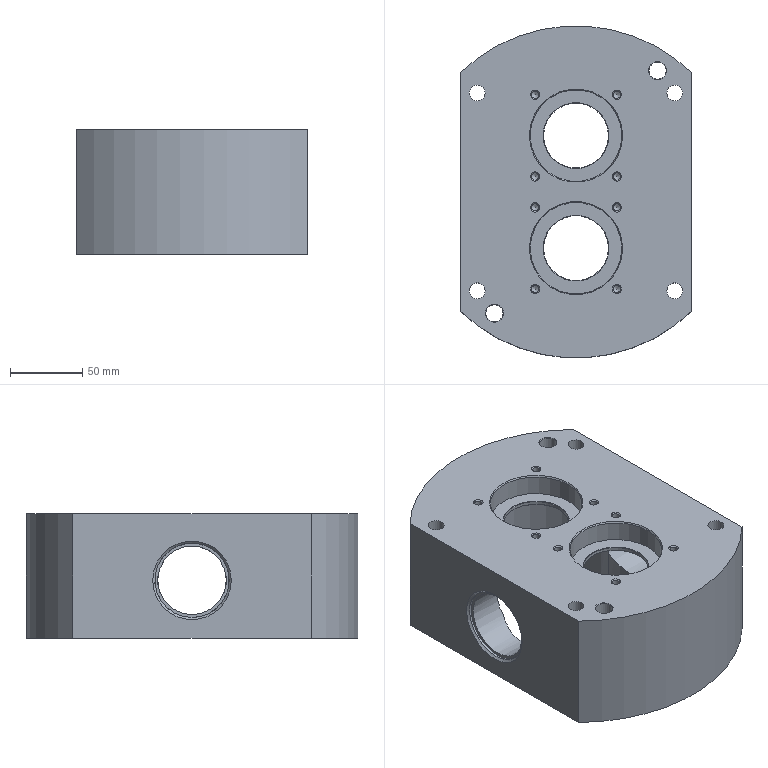NC program | NX | posted with a generic post | part box 160 x 230 x 86 mm
Lines 1 to 548 of 21365:
N10 G17 G21 G94 G90
(FLOOR_WALL_COPY_1 , TOOL : D50)
N12 T02 M6
N14 G54
N16 G17 G0 G90 X-153. Y89.997 B0. C0. S1200 M3
N18 G43 Z30. H2
N20 Z12.658
N22 G94 G1 Z9.658 F1000.
N24 X-150.
N26 X150. F2000.
N28 Y49.998
N30 X-150.
N32 Y9.999
N34 X150.
N36 Y-30.001
N38 X-150.
N40 Y-65.341
N42 Y-70.
N44 X150.
N46 X153.
N48 Z12.658
N50 G0 Z30.
N52 X-153. Y89.997
N54 Z12.317
N56 G1 Z9.317 F1000.
N58 X-150.
N60 X150. F2000.
N62 Y49.998
N64 X-150.
N66 Y9.999
N68 X150.
N70 Y-30.001
N72 X-150.
N74 Y-65.341
N76 Y-70.
N78 X150.
N80 X153.
N82 Z12.317
N84 G0 Z30.
N86 X-153. Y89.997
N88 Z11.976
N90 G1 Z8.976 F1000.
N92 X-150.
N94 X150. F2000.
N96 Y49.998
N98 X-150.
N100 Y9.999
N102 X150.
N104 Y-30.001
N106 X-150.
N108 Y-65.341
N110 Y-70.
N112 X150.
N114 X153.
N116 Z11.976
N118 G0 Z30.
N120 X-153. Y89.997
N122 Z11.634
N124 G1 Z8.634 F1000.
N126 X-150.
N128 X150. F2000.
N130 Y49.998
N132 X-150.
N134 Y9.999
N136 X150.
N138 Y-30.001
N140 X-150.
N142 Y-65.341
N144 Y-70.
N146 X150.
N148 X153.
N150 Z11.634
N152 G0 Z30.
N154 X-153. Y89.997
N156 Z11.293
N158 G1 Z8.293 F1000.
N160 X-150.
N162 X150. F2000.
N164 Y49.998
N166 X-150.
N168 Y9.999
N170 X150.
N172 Y-30.001
N174 X-150.
N176 Y-65.341
N178 Y-70.
N180 X150.
N182 X153.
N184 Z11.293
N186 G0 Z30.
N188 X-153. Y89.997
N190 Z10.951
N192 G1 Z7.951 F1000.
N194 X-150.
N196 X150. F2000.
N198 Y49.998
N200 X-150.
N202 Y9.999
N204 X150.
N206 Y-30.001
N208 X-150.
N210 Y-65.341
N212 Y-70.
N214 X150.
N216 X153.
N218 Z10.951
N220 G0 Z30.
N222 X-153. Y89.997
N224 Z10.61
N226 G1 Z7.61 F1000.
N228 X-150.
N230 X150. F2000.
N232 Y49.998
N234 X-150.
N236 Y9.999
N238 X150.
N240 Y-30.001
N242 X-150.
N244 Y-65.341
N246 Y-70.
N248 X150.
N250 X153.
N252 Z10.61
N254 G0 Z30.
N256 X-153. Y89.997
N258 Z10.269
N260 G1 Z7.269 F1000.
N262 X-150.
N264 X150. F2000.
N266 Y49.998
N268 X-150.
N270 Y9.999
N272 X150.
N274 Y-30.001
N276 X-150.
N278 Y-65.341
N280 Y-70.
N282 X150.
N284 X153.
N286 Z10.269
N288 G0 Z30.
N290 X-153. Y89.997
N292 Z9.927
N294 G1 Z6.927 F1000.
N296 X-150.
N298 X150. F2000.
N300 Y49.998
N302 X-150.
N304 Y9.999
N306 X150.
N308 Y-30.001
N310 X-150.
N312 Y-65.341
N314 Y-70.
N316 X150.
N318 X153.
N320 Z9.927
N322 G0 Z30.
N324 X-153. Y89.997
N326 Z9.586
N328 G1 Z6.586 F1000.
N330 X-150.
N332 X150. F2000.
N334 Y49.998
N336 X-150.
N338 Y9.999
N340 X150.
N342 Y-30.001
N344 X-150.
N346 Y-65.341
N348 Y-70.
N350 X150.
N352 X153.
N354 Z9.586
N356 G0 Z30.
N358 X-153. Y89.997
N360 Z9.245
N362 G1 Z6.245 F1000.
N364 X-150.
N366 X150. F2000.
N368 Y49.998
N370 X-150.
N372 Y9.999
N374 X150.
N376 Y-30.001
N378 X-150.
N380 Y-65.341
N382 Y-70.
N384 X150.
N386 X153.
N388 Z9.245
N390 G0 Z30.
N392 X-153. Y89.997
N394 Z8.903
N396 G1 Z5.903 F1000.
N398 X-150.
N400 X150. F2000.
N402 Y49.998
N404 X-150.
N406 Y9.999
N408 X150.
N410 Y-30.001
N412 X-150.
N414 Y-65.341
N416 Y-70.
N418 X150.
N420 X153.
N422 Z8.903
N424 G0 Z30.
N426 X-153. Y89.997
N428 Z8.562
N430 G1 Z5.562 F1000.
N432 X-150.
N434 X150. F2000.
N436 Y49.998
N438 X-150.
N440 Y9.999
N442 X150.
N444 Y-30.001
N446 X-150.
N448 Y-65.341
N450 Y-70.
N452 X150.
N454 X153.
N456 Z8.562
N458 G0 Z30.
N460 X-153. Y89.997
N462 Z8.221
N464 G1 Z5.221 F1000.
N466 X-150.
N468 X150. F2000.
N470 Y49.998
N472 X-150.
N474 Y9.999
N476 X150.
N478 Y-30.001
N480 X-150.
N482 Y-65.341
N484 Y-70.
N486 X150.
N488 X153.
N490 Z8.221
N492 G0 Z30.
N494 X-153. Y89.997
N496 Z7.879
N498 G1 Z4.879 F1000.
N500 X-150.
N502 X150. F2000.
N504 Y49.998
N506 X-150.
N508 Y9.999
N510 X150.
N512 Y-30.001
N514 X-150.
N516 Y-65.341
N518 Y-70.
N520 X150.
N522 X153.
N524 Z7.879
N526 G0 Z30.
N528 X-153. Y89.997
N530 Z7.538
N532 G1 Z4.538 F1000.
N534 X-150.
N536 X150. F2000.
N538 Y49.998
N540 X-150.
N542 Y9.999
N544 X150.
N546 Y-30.001
N548 X-150.
N550 Y-65.341
N552 Y-70.
N554 X150.
N556 X153.
N558 Z7.538
N560 G0 Z30.
N562 X-153. Y89.997
N564 Z7.196
N566 G1 Z4.196 F1000.
N568 X-150.
N570 X150. F2000.
N572 Y49.998
N574 X-150.
N576 Y9.999
N578 X150.
N580 Y-30.001
N582 X-150.
N584 Y-65.341
N586 Y-70.
N588 X150.
N590 X153.
N592 Z7.196
N594 G0 Z30.
N596 X-153. Y89.997
N598 Z6.855
N600 G1 Z3.855 F1000.
N602 X-150.
N604 X150. F2000.
N606 Y49.998
N608 X-150.
N610 Y9.999
N612 X150.
N614 Y-30.001
N616 X-150.
N618 Y-65.341
N620 Y-70.
N622 X150.
N624 X153.
N626 Z6.855
N628 G0 Z30.
N630 X-153. Y89.997
N632 Z6.514
N634 G1 Z3.514 F1000.
N636 X-150.
N638 X150. F2000.
N640 Y49.998
N642 X-150.
N644 Y9.999
N646 X150.
N648 Y-30.001
N650 X-150.
N652 Y-65.341
N654 Y-70.
N656 X150.
N658 X153.
N660 Z6.514
N662 G0 Z30.
N664 X-153. Y89.997
N666 Z6.172
N668 G1 Z3.172 F1000.
N670 X-150.
N672 X150. F2000.
N674 Y49.998
N676 X-150.
N678 Y9.999
N680 X150.
N682 Y-30.001
N684 X-150.
N686 Y-65.341
N688 Y-70.
N690 X150.
N692 X153.
N694 Z6.172
N696 G0 Z30.
N698 X-153. Y89.997
N700 Z5.831
N702 G1 Z2.831 F1000.
N704 X-150.
N706 X150. F2000.
N708 Y49.998
N710 X-150.
N712 Y9.999
N714 X150.
N716 Y-30.001
N718 X-150.
N720 Y-65.341
N722 Y-70.
N724 X150.
N726 X153.
N728 Z5.831
N730 G0 Z30.
N732 X-153. Y89.997
N734 Z5.49
N736 G1 Z2.49 F1000.
N738 X-150.
N740 X150. F2000.
N742 Y49.998
N744 X-150.
N746 Y9.999
N748 X150.
N750 Y-30.001
N752 X-150.
N754 Y-65.341
N756 Y-70.
N758 X150.
N760 X153.
N762 Z5.49
N764 G0 Z30.
N766 X-153. Y89.997
N768 Z5.148
N770 G1 Z2.148 F1000.
N772 X-150.
N774 X150. F2000.
N776 Y49.998
N778 X-150.
N780 Y9.999
N782 X150.
N784 Y-30.001
N786 X-150.
N788 Y-70.
N790 X150.
N792 X153.
N794 Z5.148
N796 G0 Z30.
N798 X-153. Y89.997
N800 Z4.807
N802 G1 Z1.807 F1000.
N804 X-150.
N806 X150. F2000.
N808 Y49.998
N810 X-150.
N812 Y9.999
N814 X150.
N816 Y-30.001
N818 X-150.
N820 Y-70.
N822 X150.
N824 X153.
N826 Z4.807
N828 G0 Z30.
N830 X-153. Y89.997
N832 Z4.465
N834 G1 Z1.465 F1000.
N836 X-150.
N838 X150. F2000.
N840 Y49.998
N842 X-150.
N844 Y9.999
N846 X150.
N848 Y-30.001
N850 X-150.
N852 Y-70.
N854 X150.
N856 X153.
N858 Z4.465
N860 G0 Z30.
N862 X-153. Y89.997
N864 Z4.124
N866 G1 Z1.124 F1000.
N868 X-150.
N870 X150. F2000.
N872 Y49.998
N874 X-150.
N876 Y9.999
N878 X150.
N880 Y-30.001
N882 X-150.
N884 Y-70.
N886 X150.
N888 X153.
N890 Z4.124
N892 G0 Z30.
N894 X-153. Y89.997
N896 Z3.783
N898 G1 Z0.783 F1000.
N900 X-150.
N902 X150. F2000.
N904 Y49.998
N906 X-150.
N908 Y9.999
N910 X150.
N912 Y-30.001
N914 X-150.
N916 Y-70.
N918 X150.
N920 X153.
N922 Z3.783
N924 G0 Z30.
N926 X-153. Y89.997
N928 Z3.441
N930 G1 Z0.441 F1000.
N932 X-150.
N934 X150. F2000.
N936 Y49.998
N938 X-150.
N940 Y9.999
N942 X150.
N944 Y-30.001
N946 X-150.
N948 Y-70.
N950 X150.
N952 X153.
N954 Z3.441
N956 G0 Z30.
N958 X-153. Y89.997
N960 Z3.1
N962 G1 Z0.1 F1000.
N964 X-150.
N966 X150. F2000.
N968 Y49.998
N970 X-150.
N972 Y9.999
N974 X150.
N976 Y-30.001
N978 X-150.
N980 Y-70.
N982 X150.
N984 X153.
N986 Z3.1
N988 G0 Z30.
(FLOOR_WALL_COPY_COPY , TOOL : D50)
N990 X-153. Y89.997 S2500
N992 Z3.
N994 G1 Z0. F1000.
N996 X-150.
N998 X150.
N1000 Y49.998
N1002 X-150.
N1004 Y9.999
N1006 X150.
N1008 Y-30.001
N1010 X-150.
N1012 Y-65.341
N1014 Y-70.
N1016 X150.
N1018 X153.
N1020 Z3.
N1022 G0 Z30.
N1024 M5
(DRILLING_COPY_1 , TOOL : ZXZ)
N1026 T01 M6
N1028 G54
N1030 G17 G0 G90 X105.5 Y0. B0. C0. S5000 M3
N1032 G43 Z30. H1
N1034 G94 G81 G98 Z-1. F250. R3.
N1036 X45. Y68.5
N1038 X-45.
N1040 X-105.5 Y0.
N1042 X-45. Y-68.5
N1044 X45.
N1046 G80
N1048 G0 X45. Y-68.5 Z30.
N1050 M5
(DRILLING_COPY_1_COPY , TOOL : 6.8ZT)
N1052 T16 M6
N1054 G54
N1056 G17 G0 G90 X105.5 Y0. B0. C0. S2000 M3
N1058 G43 Z30. H16
N1060 G94 G83 G98 Z-32.043 F200. Q2. R3.
N1062 X45. Y68.5
N1064 X-45.
N1066 X-105.5 Y0.
N1068 X-45. Y-68.5
N1070 X45.
N1072 G80
N1074 G0 X45. Y-68.5 Z30.
N1076 M5